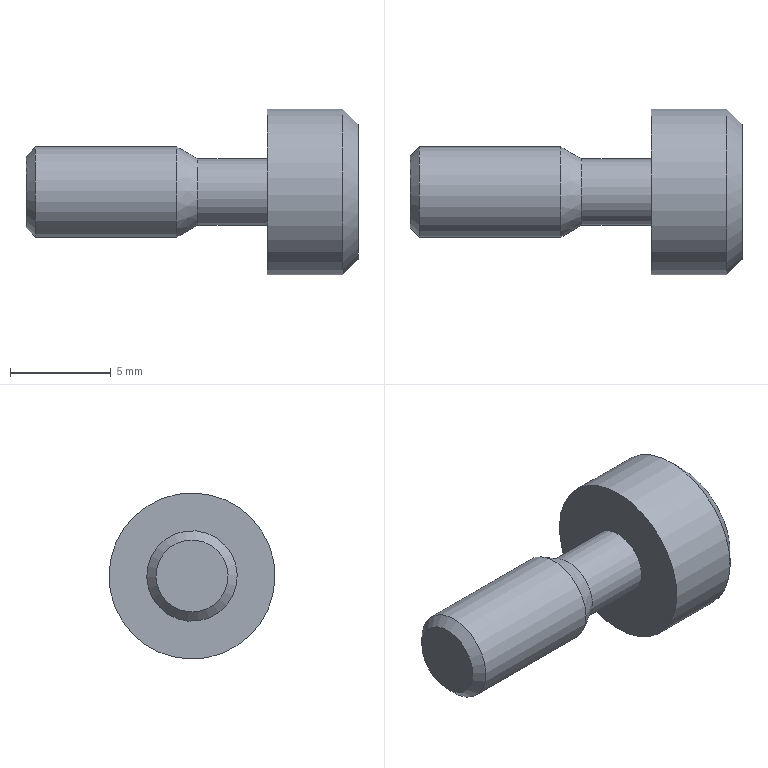Part | NX | features TAM02-M3-L8-001 2 | 1 solid | 16 faces | box 16.5 x 8.25 x 8.25 mm | volume 366.306 mm3 | plane 10 | cone 3 | cylinder 3 | commonest cylinder face diameters 3.3 x1 4.5 x1 8.25 x1
STEP:
#1=CARTESIAN_POINT('',(121.633,-41.061,-27.541));
#2=VERTEX_POINT('',#1);
#3=CARTESIAN_POINT('',(121.633,-42.7,-26.));
#4=DIRECTION('',(-1.,0.,0.));
#5=DIRECTION('',(0.,0.7285,-0.685));
#6=AXIS2_PLACEMENT_3D('',#3,#4,#5);
#7=CIRCLE('',#6,2.25);
#8=EDGE_CURVE('',#2,#2,#7,.T.);
#9=ORIENTED_EDGE('',*,*,#8,.T.);
#10=EDGE_LOOP('',(#9));
#11=FACE_BOUND('',#10,.T.);
#12=CARTESIAN_POINT('',(121.173,-41.396,-27.226));
#13=VERTEX_POINT('',#12);
#14=CARTESIAN_POINT('',(121.173,-42.7,-26.));
#15=DIRECTION('',(-1.,0.,0.));
#16=DIRECTION('',(0.,0.7285,-0.685));
#17=AXIS2_PLACEMENT_3D('',#14,#15,#16);
#18=CIRCLE('',#17,1.79);
#19=EDGE_CURVE('',#13,#13,#18,.T.);
#20=ORIENTED_EDGE('',*,*,#19,.F.);
#21=EDGE_LOOP('',(#20));
#22=FACE_BOUND('',#21,.T.);
#23=CARTESIAN_POINT('',(121.633,-42.7,-26.));
#24=DIRECTION('',(1.,0.,0.));
#25=DIRECTION('',(0.,-0.7285,0.685));
#26=AXIS2_PLACEMENT_3D('',#23,#24,#25);
#27=CONICAL_SURFACE('',#26,2.25,0.7854);
#28=ADVANCED_FACE('',(#11,#22),#27,.T.);
#29=ORIENTED_EDGE('',*,*,#8,.F.);
#30=EDGE_LOOP('',(#29));
#31=FACE_BOUND('',#30,.T.);
#32=CARTESIAN_POINT('',(128.673,-44.339,-24.459));
#33=VERTEX_POINT('',#32);
#34=CARTESIAN_POINT('',(128.673,-42.7,-26.));
#35=DIRECTION('',(1.,0.,0.));
#36=DIRECTION('',(0.,-0.7285,0.685));
#37=AXIS2_PLACEMENT_3D('',#34,#35,#36);
#38=CIRCLE('',#37,2.25);
#39=EDGE_CURVE('',#33,#33,#38,.F.);
#40=ORIENTED_EDGE('',*,*,#39,.T.);
#41=EDGE_LOOP('',(#40));
#42=FACE_BOUND('',#41,.T.);
#43=CARTESIAN_POINT('',(121.173,-42.7,-26.));
#44=DIRECTION('',(-1.,0.,0.));
#45=DIRECTION('',(0.,0.7285,-0.685));
#46=AXIS2_PLACEMENT_3D('',#43,#44,#45);
#47=CYLINDRICAL_SURFACE('',#46,2.25);
#48=ADVANCED_FACE('',(#31,#42),#47,.T.);
#49=ORIENTED_EDGE('',*,*,#39,.F.);
#50=EDGE_LOOP('',(#49));
#51=FACE_BOUND('',#50,.T.);
#52=CARTESIAN_POINT('',(129.713,-43.902,-24.87));
#53=VERTEX_POINT('',#52);
#54=CARTESIAN_POINT('',(129.713,-42.7,-26.));
#55=DIRECTION('',(1.,0.,0.));
#56=DIRECTION('',(0.,-0.7285,0.685));
#57=AXIS2_PLACEMENT_3D('',#54,#55,#56);
#58=CIRCLE('',#57,1.65);
#59=EDGE_CURVE('',#53,#53,#58,.F.);
#60=ORIENTED_EDGE('',*,*,#59,.T.);
#61=EDGE_LOOP('',(#60));
#62=FACE_BOUND('',#61,.T.);
#63=CARTESIAN_POINT('',(129.713,-42.7,-26.));
#64=DIRECTION('',(-1.,0.,0.));
#65=DIRECTION('',(0.,0.7285,-0.685));
#66=AXIS2_PLACEMENT_3D('',#63,#64,#65);
#67=CONICAL_SURFACE('',#66,1.65,0.5236);
#68=ADVANCED_FACE('',(#51,#62),#67,.T.);
#69=ORIENTED_EDGE('',*,*,#59,.F.);
#70=EDGE_LOOP('',(#69));
#71=FACE_BOUND('',#70,.T.);
#72=CARTESIAN_POINT('',(133.173,-43.902,-24.87));
#73=VERTEX_POINT('',#72);
#74=CARTESIAN_POINT('',(133.173,-42.7,-26.));
#75=DIRECTION('',(1.,0.,0.));
#76=DIRECTION('',(0.,-0.7285,0.685));
#77=AXIS2_PLACEMENT_3D('',#74,#75,#76);
#78=CIRCLE('',#77,1.65);
#79=EDGE_CURVE('',#73,#73,#78,.F.);
#80=ORIENTED_EDGE('',*,*,#79,.T.);
#81=EDGE_LOOP('',(#80));
#82=FACE_BOUND('',#81,.T.);
#83=CARTESIAN_POINT('',(121.173,-42.7,-26.));
#84=DIRECTION('',(-1.,0.,0.));
#85=DIRECTION('',(0.,0.7285,-0.685));
#86=AXIS2_PLACEMENT_3D('',#83,#84,#85);
#87=CYLINDRICAL_SURFACE('',#86,1.65);
#88=ADVANCED_FACE('',(#71,#82),#87,.T.);
#89=CARTESIAN_POINT('',(133.173,-45.705,-23.174));
#90=VERTEX_POINT('',#89);
#91=CARTESIAN_POINT('',(133.173,-42.7,-26.));
#92=DIRECTION('',(1.,0.,0.));
#93=DIRECTION('',(0.,-0.7285,0.685));
#94=AXIS2_PLACEMENT_3D('',#91,#92,#93);
#95=CIRCLE('',#94,4.125);
#96=EDGE_CURVE('',#90,#90,#95,.F.);
#97=ORIENTED_EDGE('',*,*,#96,.F.);
#98=EDGE_LOOP('',(#97));
#99=FACE_BOUND('',#98,.T.);
#100=CARTESIAN_POINT('',(136.923,-45.705,-23.174));
#101=VERTEX_POINT('',#100);
#102=CARTESIAN_POINT('',(136.923,-42.7,-26.));
#103=DIRECTION('',(1.,0.,0.));
#104=DIRECTION('',(0.,-0.7285,0.685));
#105=AXIS2_PLACEMENT_3D('',#102,#103,#104);
#106=CIRCLE('',#105,4.125);
#107=EDGE_CURVE('',#101,#101,#106,.F.);
#108=ORIENTED_EDGE('',*,*,#107,.T.);
#109=EDGE_LOOP('',(#108));
#110=FACE_BOUND('',#109,.T.);
#111=CARTESIAN_POINT('',(121.173,-42.7,-26.));
#112=DIRECTION('',(-1.,0.,0.));
#113=DIRECTION('',(0.,0.7285,-0.685));
#114=AXIS2_PLACEMENT_3D('',#111,#112,#113);
#115=CYLINDRICAL_SURFACE('',#114,4.125);
#116=ADVANCED_FACE('',(#99,#110),#115,.T.);
#117=ORIENTED_EDGE('',*,*,#107,.F.);
#118=EDGE_LOOP('',(#117));
#119=FACE_BOUND('',#118,.T.);
#120=CARTESIAN_POINT('',(137.673,-45.159,-23.688));
#121=VERTEX_POINT('',#120);
#122=CARTESIAN_POINT('',(137.673,-42.7,-26.));
#123=DIRECTION('',(1.,0.,0.));
#124=DIRECTION('',(0.,-0.7285,0.685));
#125=AXIS2_PLACEMENT_3D('',#122,#123,#124);
#126=CIRCLE('',#125,3.375);
#127=EDGE_CURVE('',#121,#121,#126,.F.);
#128=ORIENTED_EDGE('',*,*,#127,.T.);
#129=EDGE_LOOP('',(#128));
#130=FACE_BOUND('',#129,.T.);
#131=CARTESIAN_POINT('',(137.673,-42.7,-26.));
#132=DIRECTION('',(-1.,0.,0.));
#133=DIRECTION('',(0.,0.7285,-0.685));
#134=AXIS2_PLACEMENT_3D('',#131,#132,#133);
#135=CONICAL_SURFACE('',#134,3.375,0.7854);
#136=ADVANCED_FACE('',(#119,#130),#135,.T.);
#137=ORIENTED_EDGE('',*,*,#127,.F.);
#138=EDGE_LOOP('',(#137));
#139=FACE_BOUND('',#138,.T.);
#140=CARTESIAN_POINT('',(137.673,-40.592,-26.496));
#141=VERTEX_POINT('',#140);
#142=CARTESIAN_POINT('',(137.673,-42.076,-28.073));
#143=VERTEX_POINT('',#142);
#144=CARTESIAN_POINT('',(137.673,-42.076,-28.073));
#145=DIRECTION('',(0.,0.685,0.7285));
#146=VECTOR('',#145,1000.);
#147=LINE('',#144,#146);
#148=EDGE_CURVE('',#141,#143,#147,.F.);
#149=ORIENTED_EDGE('',*,*,#148,.T.);
#150=CARTESIAN_POINT('',(137.673,-44.183,-27.577));
#151=VERTEX_POINT('',#150);
#152=CARTESIAN_POINT('',(137.673,-44.183,-27.577));
#153=DIRECTION('',(0.,0.9734,-0.229));
#154=VECTOR('',#153,1000.);
#155=LINE('',#152,#154);
#156=EDGE_CURVE('',#143,#151,#155,.F.);
#157=ORIENTED_EDGE('',*,*,#156,.T.);
#158=CARTESIAN_POINT('',(137.673,-44.808,-25.504));
#159=VERTEX_POINT('',#158);
#160=CARTESIAN_POINT('',(137.673,-44.808,-25.504));
#161=DIRECTION('',(0.,0.2884,-0.9575));
#162=VECTOR('',#161,1000.);
#163=LINE('',#160,#162);
#164=EDGE_CURVE('',#151,#159,#163,.F.);
#165=ORIENTED_EDGE('',*,*,#164,.T.);
#166=CARTESIAN_POINT('',(137.673,-43.324,-23.927));
#167=VERTEX_POINT('',#166);
#168=CARTESIAN_POINT('',(137.673,-43.324,-23.927));
#169=DIRECTION('',(0.,-0.685,-0.7285));
#170=VECTOR('',#169,1000.);
#171=LINE('',#168,#170);
#172=EDGE_CURVE('',#159,#167,#171,.F.);
#173=ORIENTED_EDGE('',*,*,#172,.T.);
#174=CARTESIAN_POINT('',(137.673,-41.217,-24.423));
#175=VERTEX_POINT('',#174);
#176=CARTESIAN_POINT('',(137.673,-41.217,-24.423));
#177=DIRECTION('',(0.,-0.9734,0.229));
#178=VECTOR('',#177,1000.);
#179=LINE('',#176,#178);
#180=EDGE_CURVE('',#167,#175,#179,.F.);
#181=ORIENTED_EDGE('',*,*,#180,.T.);
#182=CARTESIAN_POINT('',(137.673,-40.592,-26.496));
#183=DIRECTION('',(0.,-0.2884,0.9575));
#184=VECTOR('',#183,1000.);
#185=LINE('',#182,#184);
#186=EDGE_CURVE('',#175,#141,#185,.F.);
#187=ORIENTED_EDGE('',*,*,#186,.T.);
#188=EDGE_LOOP('',(#149,#157,#165,#173,#181,#187));
#189=FACE_BOUND('',#188,.T.);
#190=CARTESIAN_POINT('',(137.673,-42.7,-26.));
#191=DIRECTION('',(-1.,0.,0.));
#192=DIRECTION('',(0.,0.7285,-0.685));
#193=AXIS2_PLACEMENT_3D('',#190,#191,#192);
#194=PLANE('',#193);
#195=ADVANCED_FACE('',(#139,#189),#194,.F.);
#196=ORIENTED_EDGE('',*,*,#79,.F.);
#197=EDGE_LOOP('',(#196));
#198=FACE_BOUND('',#197,.T.);
#199=ORIENTED_EDGE('',*,*,#96,.T.);
#200=EDGE_LOOP('',(#199));
#201=FACE_BOUND('',#200,.T.);
#202=CARTESIAN_POINT('',(133.173,-45.526,-29.005));
#203=DIRECTION('',(1.,0.,0.));
#204=DIRECTION('',(0.,-0.7285,0.685));
#205=AXIS2_PLACEMENT_3D('',#202,#203,#204);
#206=PLANE('',#205);
#207=ADVANCED_FACE('',(#198,#201),#206,.F.);
#208=ORIENTED_EDGE('',*,*,#19,.T.);
#209=EDGE_LOOP('',(#208));
#210=FACE_BOUND('',#209,.T.);
#211=CARTESIAN_POINT('',(121.173,-43.926,-27.304));
#212=DIRECTION('',(1.,0.,0.));
#213=DIRECTION('',(0.,-0.7285,0.685));
#214=AXIS2_PLACEMENT_3D('',#211,#212,#213);
#215=PLANE('',#214);
#216=ADVANCED_FACE('',(#210),#215,.F.);
#217=ORIENTED_EDGE('',*,*,#148,.F.);
#218=CARTESIAN_POINT('',(135.423,-40.592,-26.496));
#219=VERTEX_POINT('',#218);
#220=CARTESIAN_POINT('',(135.423,-40.592,-26.496));
#221=DIRECTION('',(1.,0.,0.));
#222=VECTOR('',#221,1000.);
#223=LINE('',#220,#222);
#224=EDGE_CURVE('',#141,#219,#223,.F.);
#225=ORIENTED_EDGE('',*,*,#224,.T.);
#226=CARTESIAN_POINT('',(135.423,-42.076,-28.073));
#227=VERTEX_POINT('',#226);
#228=CARTESIAN_POINT('',(135.423,-42.076,-28.073));
#229=DIRECTION('',(0.,0.685,0.7285));
#230=VECTOR('',#229,1000.);
#231=LINE('',#228,#230);
#232=EDGE_CURVE('',#219,#227,#231,.F.);
#233=ORIENTED_EDGE('',*,*,#232,.T.);
#234=CARTESIAN_POINT('',(135.423,-42.076,-28.073));
#235=DIRECTION('',(1.,0.,0.));
#236=VECTOR('',#235,1000.);
#237=LINE('',#234,#236);
#238=EDGE_CURVE('',#143,#227,#237,.F.);
#239=ORIENTED_EDGE('',*,*,#238,.F.);
#240=EDGE_LOOP('',(#217,#225,#233,#239));
#241=FACE_BOUND('',#240,.T.);
#242=CARTESIAN_POINT('',(135.423,-42.076,-28.073));
#243=DIRECTION('',(0.,-0.7285,0.685));
#244=DIRECTION('',(-1.,0.,0.));
#245=AXIS2_PLACEMENT_3D('',#242,#243,#244);
#246=PLANE('',#245);
#247=ADVANCED_FACE('',(#241),#246,.T.);
#248=ORIENTED_EDGE('',*,*,#186,.F.);
#249=CARTESIAN_POINT('',(135.423,-41.217,-24.423));
#250=VERTEX_POINT('',#249);
#251=CARTESIAN_POINT('',(135.423,-41.217,-24.423));
#252=DIRECTION('',(1.,0.,0.));
#253=VECTOR('',#252,1000.);
#254=LINE('',#251,#253);
#255=EDGE_CURVE('',#175,#250,#254,.F.);
#256=ORIENTED_EDGE('',*,*,#255,.T.);
#257=CARTESIAN_POINT('',(135.423,-40.592,-26.496));
#258=DIRECTION('',(0.,-0.2884,0.9575));
#259=VECTOR('',#258,1000.);
#260=LINE('',#257,#259);
#261=EDGE_CURVE('',#250,#219,#260,.F.);
#262=ORIENTED_EDGE('',*,*,#261,.T.);
#263=ORIENTED_EDGE('',*,*,#224,.F.);
#264=EDGE_LOOP('',(#248,#256,#262,#263));
#265=FACE_BOUND('',#264,.T.);
#266=CARTESIAN_POINT('',(135.423,-40.592,-26.496));
#267=DIRECTION('',(0.,-0.9575,-0.2884));
#268=DIRECTION('',(0.,-0.2884,0.9575));
#269=AXIS2_PLACEMENT_3D('',#266,#267,#268);
#270=PLANE('',#269);
#271=ADVANCED_FACE('',(#265),#270,.T.);
#272=ORIENTED_EDGE('',*,*,#180,.F.);
#273=CARTESIAN_POINT('',(135.423,-43.324,-23.927));
#274=VERTEX_POINT('',#273);
#275=CARTESIAN_POINT('',(135.423,-43.324,-23.927));
#276=DIRECTION('',(1.,0.,0.));
#277=VECTOR('',#276,1000.);
#278=LINE('',#275,#277);
#279=EDGE_CURVE('',#167,#274,#278,.F.);
#280=ORIENTED_EDGE('',*,*,#279,.T.);
#281=CARTESIAN_POINT('',(135.423,-41.217,-24.423));
#282=DIRECTION('',(0.,-0.9734,0.229));
#283=VECTOR('',#282,1000.);
#284=LINE('',#281,#283);
#285=EDGE_CURVE('',#274,#250,#284,.F.);
#286=ORIENTED_EDGE('',*,*,#285,.T.);
#287=ORIENTED_EDGE('',*,*,#255,.F.);
#288=EDGE_LOOP('',(#272,#280,#286,#287));
#289=FACE_BOUND('',#288,.T.);
#290=CARTESIAN_POINT('',(135.423,-41.217,-24.423));
#291=DIRECTION('',(0.,-0.229,-0.9734));
#292=DIRECTION('',(0.,-0.9734,0.229));
#293=AXIS2_PLACEMENT_3D('',#290,#291,#292);
#294=PLANE('',#293);
#295=ADVANCED_FACE('',(#289),#294,.T.);
#296=ORIENTED_EDGE('',*,*,#172,.F.);
#297=CARTESIAN_POINT('',(135.423,-44.808,-25.504));
#298=VERTEX_POINT('',#297);
#299=CARTESIAN_POINT('',(135.423,-44.808,-25.504));
#300=DIRECTION('',(1.,0.,0.));
#301=VECTOR('',#300,1000.);
#302=LINE('',#299,#301);
#303=EDGE_CURVE('',#159,#298,#302,.F.);
#304=ORIENTED_EDGE('',*,*,#303,.T.);
#305=CARTESIAN_POINT('',(135.423,-43.324,-23.927));
#306=DIRECTION('',(0.,-0.685,-0.7285));
#307=VECTOR('',#306,1000.);
#308=LINE('',#305,#307);
#309=EDGE_CURVE('',#298,#274,#308,.F.);
#310=ORIENTED_EDGE('',*,*,#309,.T.);
#311=ORIENTED_EDGE('',*,*,#279,.F.);
#312=EDGE_LOOP('',(#296,#304,#310,#311));
#313=FACE_BOUND('',#312,.T.);
#314=CARTESIAN_POINT('',(135.423,-43.324,-23.927));
#315=DIRECTION('',(0.,0.7285,-0.685));
#316=DIRECTION('',(1.,0.,0.));
#317=AXIS2_PLACEMENT_3D('',#314,#315,#316);
#318=PLANE('',#317);
#319=ADVANCED_FACE('',(#313),#318,.T.);
#320=ORIENTED_EDGE('',*,*,#164,.F.);
#321=CARTESIAN_POINT('',(135.423,-44.183,-27.577));
#322=VERTEX_POINT('',#321);
#323=CARTESIAN_POINT('',(135.423,-44.183,-27.577));
#324=DIRECTION('',(1.,0.,0.));
#325=VECTOR('',#324,1000.);
#326=LINE('',#323,#325);
#327=EDGE_CURVE('',#151,#322,#326,.F.);
#328=ORIENTED_EDGE('',*,*,#327,.T.);
#329=CARTESIAN_POINT('',(135.423,-44.808,-25.504));
#330=DIRECTION('',(0.,0.2884,-0.9575));
#331=VECTOR('',#330,1000.);
#332=LINE('',#329,#331);
#333=EDGE_CURVE('',#322,#298,#332,.F.);
#334=ORIENTED_EDGE('',*,*,#333,.T.);
#335=ORIENTED_EDGE('',*,*,#303,.F.);
#336=EDGE_LOOP('',(#320,#328,#334,#335));
#337=FACE_BOUND('',#336,.T.);
#338=CARTESIAN_POINT('',(135.423,-44.808,-25.504));
#339=DIRECTION('',(0.,0.9575,0.2884));
#340=DIRECTION('',(0.,0.2884,-0.9575));
#341=AXIS2_PLACEMENT_3D('',#338,#339,#340);
#342=PLANE('',#341);
#343=ADVANCED_FACE('',(#337),#342,.T.);
#344=ORIENTED_EDGE('',*,*,#156,.F.);
#345=ORIENTED_EDGE('',*,*,#238,.T.);
#346=CARTESIAN_POINT('',(135.423,-44.183,-27.577));
#347=DIRECTION('',(0.,0.9734,-0.229));
#348=VECTOR('',#347,1000.);
#349=LINE('',#346,#348);
#350=EDGE_CURVE('',#227,#322,#349,.F.);
#351=ORIENTED_EDGE('',*,*,#350,.T.);
#352=ORIENTED_EDGE('',*,*,#327,.F.);
#353=EDGE_LOOP('',(#344,#345,#351,#352));
#354=FACE_BOUND('',#353,.T.);
#355=CARTESIAN_POINT('',(135.423,-44.183,-27.577));
#356=DIRECTION('',(0.,0.229,0.9734));
#357=DIRECTION('',(0.,0.9734,-0.229));
#358=AXIS2_PLACEMENT_3D('',#355,#356,#357);
#359=PLANE('',#358);
#360=ADVANCED_FACE('',(#354),#359,.T.);
#361=ORIENTED_EDGE('',*,*,#232,.F.);
#362=ORIENTED_EDGE('',*,*,#261,.F.);
#363=ORIENTED_EDGE('',*,*,#285,.F.);
#364=ORIENTED_EDGE('',*,*,#309,.F.);
#365=ORIENTED_EDGE('',*,*,#333,.F.);
#366=ORIENTED_EDGE('',*,*,#350,.F.);
#367=EDGE_LOOP('',(#361,#362,#363,#364,#365,#366));
#368=FACE_BOUND('',#367,.T.);
#369=CARTESIAN_POINT('',(135.423,-42.7,-26.));
#370=DIRECTION('',(-1.,0.,0.));
#371=DIRECTION('',(0.,0.7285,-0.685));
#372=AXIS2_PLACEMENT_3D('',#369,#370,#371);
#373=PLANE('',#372);
#374=ADVANCED_FACE('',(#368),#373,.F.);
#375=CLOSED_SHELL('',(#28,#48,#68,#88,#116,#136,#195,#207,#216,#247,#271,#295,#319,#343,#360,#374));
#376=MANIFOLD_SOLID_BREP('',#375);
#377=(LENGTH_UNIT()NAMED_UNIT(*)SI_UNIT(.MILLI.,.METRE.));
#378=UNCERTAINTY_MEASURE_WITH_UNIT(LENGTH_MEASURE(0.00001),#377,'','');
#379=(NAMED_UNIT(*)PLANE_ANGLE_UNIT()SI_UNIT($,.RADIAN.));
#380=(NAMED_UNIT(*)SI_UNIT($,.STERADIAN.)SOLID_ANGLE_UNIT());
#381=(GEOMETRIC_REPRESENTATION_CONTEXT(3)GLOBAL_UNCERTAINTY_ASSIGNED_CONTEXT((#378))GLOBAL_UNIT_ASSIGNED_CONTEXT((#377,#379,#380))REPRESENTATION_CONTEXT('',''));
#382=ADVANCED_BREP_SHAPE_REPRESENTATION('',(#376),#381);